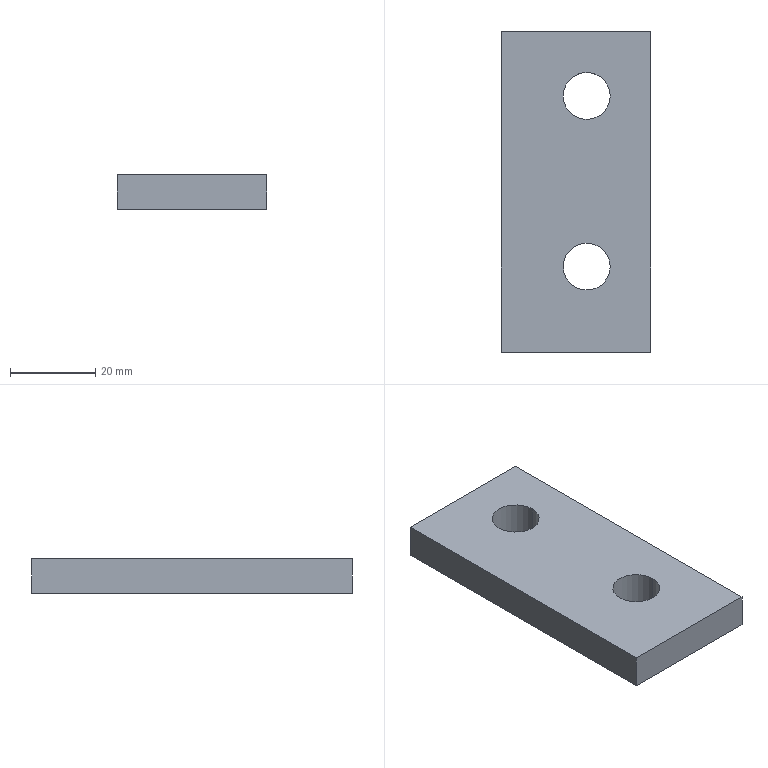Part | SolidWorks | features BaseBody 1 | 1 solid | 10 faces | box 35 x 75 x 8 mm | volume 19479 mm3 | plane 6 | cylinder 4 | commonest cylinder face diameters 11 x4
STEP:
#1=CARTESIAN_POINT('',(-3.,22.5,8.));
#2=VERTEX_POINT('',#1);
#3=CARTESIAN_POINT('',(8.,22.5,8.));
#4=VERTEX_POINT('',#3);
#5=CARTESIAN_POINT('',(2.5,22.5,8.));
#6=DIRECTION('',(0.,0.,1.));
#7=DIRECTION('',(1.,0.,0.));
#8=AXIS2_PLACEMENT_3D('',#5,#6,#7);
#9=CIRCLE('',#8,5.5);
#10=EDGE_CURVE('',#2,#4,#9,.T.);
#11=ORIENTED_EDGE('',*,*,#10,.T.);
#12=CARTESIAN_POINT('',(8.,22.5,0.));
#13=VERTEX_POINT('',#12);
#14=CARTESIAN_POINT('',(8.,22.5,0.));
#15=DIRECTION('',(0.,0.,-1.));
#16=VECTOR('',#15,1000.);
#17=LINE('',#14,#16);
#18=EDGE_CURVE('',#4,#13,#17,.T.);
#19=ORIENTED_EDGE('',*,*,#18,.T.);
#20=CARTESIAN_POINT('',(-3.,22.5,0.));
#21=VERTEX_POINT('',#20);
#22=CARTESIAN_POINT('',(2.5,22.5,0.));
#23=DIRECTION('',(0.,0.,-1.));
#24=DIRECTION('',(-1.,0.,0.));
#25=AXIS2_PLACEMENT_3D('',#22,#23,#24);
#26=CIRCLE('',#25,5.5);
#27=EDGE_CURVE('',#13,#21,#26,.T.);
#28=ORIENTED_EDGE('',*,*,#27,.T.);
#29=CARTESIAN_POINT('',(-3.,22.5,0.));
#30=DIRECTION('',(0.,0.,-1.));
#31=VECTOR('',#30,1000.);
#32=LINE('',#29,#31);
#33=EDGE_CURVE('',#2,#21,#32,.T.);
#34=ORIENTED_EDGE('',*,*,#33,.F.);
#35=EDGE_LOOP('',(#11,#19,#28,#34));
#36=FACE_OUTER_BOUND('',#35,.T.);
#37=CARTESIAN_POINT('',(2.5,22.5,0.));
#38=DIRECTION('',(0.,0.,-1.));
#39=DIRECTION('',(-1.,0.,0.));
#40=AXIS2_PLACEMENT_3D('',#37,#38,#39);
#41=CYLINDRICAL_SURFACE('',#40,5.5);
#42=ADVANCED_FACE('',(#36),#41,.F.);
#43=CARTESIAN_POINT('',(-3.,-17.5,8.));
#44=VERTEX_POINT('',#43);
#45=CARTESIAN_POINT('',(8.,-17.5,8.));
#46=VERTEX_POINT('',#45);
#47=CARTESIAN_POINT('',(2.5,-17.5,8.));
#48=DIRECTION('',(0.,0.,1.));
#49=DIRECTION('',(1.,0.,0.));
#50=AXIS2_PLACEMENT_3D('',#47,#48,#49);
#51=CIRCLE('',#50,5.5);
#52=EDGE_CURVE('',#44,#46,#51,.T.);
#53=ORIENTED_EDGE('',*,*,#52,.T.);
#54=CARTESIAN_POINT('',(8.,-17.5,0.));
#55=VERTEX_POINT('',#54);
#56=CARTESIAN_POINT('',(8.,-17.5,0.));
#57=DIRECTION('',(0.,0.,-1.));
#58=VECTOR('',#57,1000.);
#59=LINE('',#56,#58);
#60=EDGE_CURVE('',#46,#55,#59,.T.);
#61=ORIENTED_EDGE('',*,*,#60,.T.);
#62=CARTESIAN_POINT('',(-3.,-17.5,0.));
#63=VERTEX_POINT('',#62);
#64=CARTESIAN_POINT('',(2.5,-17.5,0.));
#65=DIRECTION('',(0.,0.,-1.));
#66=DIRECTION('',(-1.,0.,0.));
#67=AXIS2_PLACEMENT_3D('',#64,#65,#66);
#68=CIRCLE('',#67,5.5);
#69=EDGE_CURVE('',#55,#63,#68,.T.);
#70=ORIENTED_EDGE('',*,*,#69,.T.);
#71=CARTESIAN_POINT('',(-3.,-17.5,0.));
#72=DIRECTION('',(0.,0.,-1.));
#73=VECTOR('',#72,1000.);
#74=LINE('',#71,#73);
#75=EDGE_CURVE('',#44,#63,#74,.T.);
#76=ORIENTED_EDGE('',*,*,#75,.F.);
#77=EDGE_LOOP('',(#53,#61,#70,#76));
#78=FACE_OUTER_BOUND('',#77,.T.);
#79=CARTESIAN_POINT('',(2.5,-17.5,0.));
#80=DIRECTION('',(0.,0.,-1.));
#81=DIRECTION('',(-1.,0.,0.));
#82=AXIS2_PLACEMENT_3D('',#79,#80,#81);
#83=CYLINDRICAL_SURFACE('',#82,5.5);
#84=ADVANCED_FACE('',(#78),#83,.F.);
#85=CARTESIAN_POINT('',(2.5,-17.5,0.));
#86=DIRECTION('',(0.,0.,-1.));
#87=DIRECTION('',(-1.,0.,0.));
#88=AXIS2_PLACEMENT_3D('',#85,#86,#87);
#89=CIRCLE('',#88,5.5);
#90=EDGE_CURVE('',#63,#55,#89,.T.);
#91=ORIENTED_EDGE('',*,*,#90,.F.);
#92=ORIENTED_EDGE('',*,*,#69,.F.);
#93=EDGE_LOOP('',(#91,#92));
#94=FACE_BOUND('',#93,.T.);
#95=CARTESIAN_POINT('',(2.5,22.5,0.));
#96=DIRECTION('',(0.,0.,-1.));
#97=DIRECTION('',(-1.,0.,0.));
#98=AXIS2_PLACEMENT_3D('',#95,#96,#97);
#99=CIRCLE('',#98,5.5);
#100=EDGE_CURVE('',#21,#13,#99,.T.);
#101=ORIENTED_EDGE('',*,*,#100,.F.);
#102=ORIENTED_EDGE('',*,*,#27,.F.);
#103=EDGE_LOOP('',(#101,#102));
#104=FACE_BOUND('',#103,.T.);
#105=CARTESIAN_POINT('',(17.5,-37.5,0.));
#106=VERTEX_POINT('',#105);
#107=CARTESIAN_POINT('',(17.5,37.5,0.));
#108=VERTEX_POINT('',#107);
#109=CARTESIAN_POINT('',(17.5,37.5,0.));
#110=DIRECTION('',(0.,1.,0.));
#111=VECTOR('',#110,1000.);
#112=LINE('',#109,#111);
#113=EDGE_CURVE('',#106,#108,#112,.T.);
#114=ORIENTED_EDGE('',*,*,#113,.F.);
#115=CARTESIAN_POINT('',(-17.5,-37.5,0.));
#116=VERTEX_POINT('',#115);
#117=CARTESIAN_POINT('',(-17.5,-37.5,0.));
#118=DIRECTION('',(1.,0.,0.));
#119=VECTOR('',#118,1000.);
#120=LINE('',#117,#119);
#121=EDGE_CURVE('',#116,#106,#120,.T.);
#122=ORIENTED_EDGE('',*,*,#121,.F.);
#123=CARTESIAN_POINT('',(-17.5,37.5,0.));
#124=VERTEX_POINT('',#123);
#125=CARTESIAN_POINT('',(-17.5,37.5,0.));
#126=DIRECTION('',(0.,-1.,0.));
#127=VECTOR('',#126,1000.);
#128=LINE('',#125,#127);
#129=EDGE_CURVE('',#124,#116,#128,.T.);
#130=ORIENTED_EDGE('',*,*,#129,.F.);
#131=CARTESIAN_POINT('',(-17.5,37.5,0.));
#132=DIRECTION('',(-1.,0.,0.));
#133=VECTOR('',#132,1000.);
#134=LINE('',#131,#133);
#135=EDGE_CURVE('',#108,#124,#134,.T.);
#136=ORIENTED_EDGE('',*,*,#135,.F.);
#137=EDGE_LOOP('',(#114,#122,#130,#136));
#138=FACE_OUTER_BOUND('',#137,.T.);
#139=CARTESIAN_POINT('',(0.,0.,0.));
#140=DIRECTION('',(0.,0.,1.));
#141=DIRECTION('',(1.,0.,0.));
#142=AXIS2_PLACEMENT_3D('',#139,#140,#141);
#143=PLANE('',#142);
#144=ADVANCED_FACE('',(#94,#104,#138),#143,.F.);
#145=ORIENTED_EDGE('',*,*,#52,.F.);
#146=CARTESIAN_POINT('',(2.5,-17.5,8.));
#147=DIRECTION('',(0.,0.,1.));
#148=DIRECTION('',(1.,0.,0.));
#149=AXIS2_PLACEMENT_3D('',#146,#147,#148);
#150=CIRCLE('',#149,5.5);
#151=EDGE_CURVE('',#46,#44,#150,.T.);
#152=ORIENTED_EDGE('',*,*,#151,.F.);
#153=EDGE_LOOP('',(#145,#152));
#154=FACE_BOUND('',#153,.T.);
#155=ORIENTED_EDGE('',*,*,#10,.F.);
#156=CARTESIAN_POINT('',(2.5,22.5,8.));
#157=DIRECTION('',(0.,0.,1.));
#158=DIRECTION('',(1.,0.,0.));
#159=AXIS2_PLACEMENT_3D('',#156,#157,#158);
#160=CIRCLE('',#159,5.5);
#161=EDGE_CURVE('',#4,#2,#160,.T.);
#162=ORIENTED_EDGE('',*,*,#161,.F.);
#163=EDGE_LOOP('',(#155,#162));
#164=FACE_BOUND('',#163,.T.);
#165=CARTESIAN_POINT('',(17.5,-37.5,8.));
#166=VERTEX_POINT('',#165);
#167=CARTESIAN_POINT('',(17.5,37.5,8.));
#168=VERTEX_POINT('',#167);
#169=CARTESIAN_POINT('',(17.5,37.5,8.));
#170=DIRECTION('',(0.,1.,0.));
#171=VECTOR('',#170,1000.);
#172=LINE('',#169,#171);
#173=EDGE_CURVE('',#166,#168,#172,.T.);
#174=ORIENTED_EDGE('',*,*,#173,.T.);
#175=CARTESIAN_POINT('',(-17.5,37.5,8.));
#176=VERTEX_POINT('',#175);
#177=CARTESIAN_POINT('',(-17.5,37.5,8.));
#178=DIRECTION('',(-1.,0.,0.));
#179=VECTOR('',#178,1000.);
#180=LINE('',#177,#179);
#181=EDGE_CURVE('',#168,#176,#180,.T.);
#182=ORIENTED_EDGE('',*,*,#181,.T.);
#183=CARTESIAN_POINT('',(-17.5,-37.5,8.));
#184=VERTEX_POINT('',#183);
#185=CARTESIAN_POINT('',(-17.5,37.5,8.));
#186=DIRECTION('',(0.,-1.,0.));
#187=VECTOR('',#186,1000.);
#188=LINE('',#185,#187);
#189=EDGE_CURVE('',#176,#184,#188,.T.);
#190=ORIENTED_EDGE('',*,*,#189,.T.);
#191=CARTESIAN_POINT('',(-17.5,-37.5,8.));
#192=DIRECTION('',(1.,0.,0.));
#193=VECTOR('',#192,1000.);
#194=LINE('',#191,#193);
#195=EDGE_CURVE('',#184,#166,#194,.T.);
#196=ORIENTED_EDGE('',*,*,#195,.T.);
#197=EDGE_LOOP('',(#174,#182,#190,#196));
#198=FACE_OUTER_BOUND('',#197,.T.);
#199=CARTESIAN_POINT('',(0.,0.,8.));
#200=DIRECTION('',(0.,0.,1.));
#201=DIRECTION('',(1.,0.,0.));
#202=AXIS2_PLACEMENT_3D('',#199,#200,#201);
#203=PLANE('',#202);
#204=ADVANCED_FACE('',(#154,#164,#198),#203,.T.);
#205=ORIENTED_EDGE('',*,*,#121,.T.);
#206=CARTESIAN_POINT('',(17.5,-37.5,8.));
#207=DIRECTION('',(0.,0.,-1.));
#208=VECTOR('',#207,1000.);
#209=LINE('',#206,#208);
#210=EDGE_CURVE('',#166,#106,#209,.T.);
#211=ORIENTED_EDGE('',*,*,#210,.F.);
#212=ORIENTED_EDGE('',*,*,#195,.F.);
#213=CARTESIAN_POINT('',(-17.5,-37.5,8.));
#214=DIRECTION('',(0.,0.,-1.));
#215=VECTOR('',#214,1000.);
#216=LINE('',#213,#215);
#217=EDGE_CURVE('',#184,#116,#216,.T.);
#218=ORIENTED_EDGE('',*,*,#217,.T.);
#219=EDGE_LOOP('',(#205,#211,#212,#218));
#220=FACE_OUTER_BOUND('',#219,.T.);
#221=CARTESIAN_POINT('',(-17.5,-37.5,8.));
#222=DIRECTION('',(0.,1.,0.));
#223=DIRECTION('',(1.,0.,0.));
#224=AXIS2_PLACEMENT_3D('',#221,#222,#223);
#225=PLANE('',#224);
#226=ADVANCED_FACE('',(#220),#225,.F.);
#227=ORIENTED_EDGE('',*,*,#129,.T.);
#228=ORIENTED_EDGE('',*,*,#217,.F.);
#229=ORIENTED_EDGE('',*,*,#189,.F.);
#230=CARTESIAN_POINT('',(-17.5,37.5,8.));
#231=DIRECTION('',(0.,0.,-1.));
#232=VECTOR('',#231,1000.);
#233=LINE('',#230,#232);
#234=EDGE_CURVE('',#176,#124,#233,.T.);
#235=ORIENTED_EDGE('',*,*,#234,.T.);
#236=EDGE_LOOP('',(#227,#228,#229,#235));
#237=FACE_OUTER_BOUND('',#236,.T.);
#238=CARTESIAN_POINT('',(-17.5,37.5,8.));
#239=DIRECTION('',(1.,0.,0.));
#240=DIRECTION('',(0.,1.,0.));
#241=AXIS2_PLACEMENT_3D('',#238,#239,#240);
#242=PLANE('',#241);
#243=ADVANCED_FACE('',(#237),#242,.F.);
#244=ORIENTED_EDGE('',*,*,#135,.T.);
#245=ORIENTED_EDGE('',*,*,#234,.F.);
#246=ORIENTED_EDGE('',*,*,#181,.F.);
#247=CARTESIAN_POINT('',(17.5,37.5,8.));
#248=DIRECTION('',(0.,0.,-1.));
#249=VECTOR('',#248,1000.);
#250=LINE('',#247,#249);
#251=EDGE_CURVE('',#168,#108,#250,.T.);
#252=ORIENTED_EDGE('',*,*,#251,.T.);
#253=EDGE_LOOP('',(#244,#245,#246,#252));
#254=FACE_OUTER_BOUND('',#253,.T.);
#255=CARTESIAN_POINT('',(-17.5,37.5,8.));
#256=DIRECTION('',(0.,-1.,0.));
#257=DIRECTION('',(0.,0.,-1.));
#258=AXIS2_PLACEMENT_3D('',#255,#256,#257);
#259=PLANE('',#258);
#260=ADVANCED_FACE('',(#254),#259,.F.);
#261=ORIENTED_EDGE('',*,*,#113,.T.);
#262=ORIENTED_EDGE('',*,*,#251,.F.);
#263=ORIENTED_EDGE('',*,*,#173,.F.);
#264=ORIENTED_EDGE('',*,*,#210,.T.);
#265=EDGE_LOOP('',(#261,#262,#263,#264));
#266=FACE_OUTER_BOUND('',#265,.T.);
#267=CARTESIAN_POINT('',(17.5,37.5,8.));
#268=DIRECTION('',(-1.,0.,0.));
#269=DIRECTION('',(0.,0.,1.));
#270=AXIS2_PLACEMENT_3D('',#267,#268,#269);
#271=PLANE('',#270);
#272=ADVANCED_FACE('',(#266),#271,.F.);
#273=ORIENTED_EDGE('',*,*,#60,.F.);
#274=ORIENTED_EDGE('',*,*,#151,.T.);
#275=ORIENTED_EDGE('',*,*,#75,.T.);
#276=ORIENTED_EDGE('',*,*,#90,.T.);
#277=EDGE_LOOP('',(#273,#274,#275,#276));
#278=FACE_OUTER_BOUND('',#277,.T.);
#279=CARTESIAN_POINT('',(2.5,-17.5,0.));
#280=DIRECTION('',(0.,0.,-1.));
#281=DIRECTION('',(-1.,0.,0.));
#282=AXIS2_PLACEMENT_3D('',#279,#280,#281);
#283=CYLINDRICAL_SURFACE('',#282,5.5);
#284=ADVANCED_FACE('',(#278),#283,.F.);
#285=ORIENTED_EDGE('',*,*,#18,.F.);
#286=ORIENTED_EDGE('',*,*,#161,.T.);
#287=ORIENTED_EDGE('',*,*,#33,.T.);
#288=ORIENTED_EDGE('',*,*,#100,.T.);
#289=EDGE_LOOP('',(#285,#286,#287,#288));
#290=FACE_OUTER_BOUND('',#289,.T.);
#291=CARTESIAN_POINT('',(2.5,22.5,0.));
#292=DIRECTION('',(0.,0.,-1.));
#293=DIRECTION('',(-1.,0.,0.));
#294=AXIS2_PLACEMENT_3D('',#291,#292,#293);
#295=CYLINDRICAL_SURFACE('',#294,5.5);
#296=ADVANCED_FACE('',(#290),#295,.F.);
#297=CLOSED_SHELL('',(#42,#84,#144,#204,#226,#243,#260,#272,#284,#296));
#298=MANIFOLD_SOLID_BREP('',#297);
#299=CARTESIAN_POINT('',(0.,0.,0.));
#300=DIRECTION('',(0.,0.,1.));
#301=DIRECTION('',(1.,0.,0.));
#302=AXIS2_PLACEMENT_3D('',#299,#300,#301);
#303=(LENGTH_UNIT()NAMED_UNIT(*)SI_UNIT(.MILLI.,.METRE.));
#304=UNCERTAINTY_MEASURE_WITH_UNIT(LENGTH_MEASURE(0.00001),#303,'','');
#305=(NAMED_UNIT(*)PLANE_ANGLE_UNIT()SI_UNIT($,.RADIAN.));
#306=(NAMED_UNIT(*)SI_UNIT($,.STERADIAN.)SOLID_ANGLE_UNIT());
#307=(GEOMETRIC_REPRESENTATION_CONTEXT(3)GLOBAL_UNCERTAINTY_ASSIGNED_CONTEXT((#304))GLOBAL_UNIT_ASSIGNED_CONTEXT((#303,#305,#306))REPRESENTATION_CONTEXT('',''));
#308=ADVANCED_BREP_SHAPE_REPRESENTATION('',(#298,#302),#307);